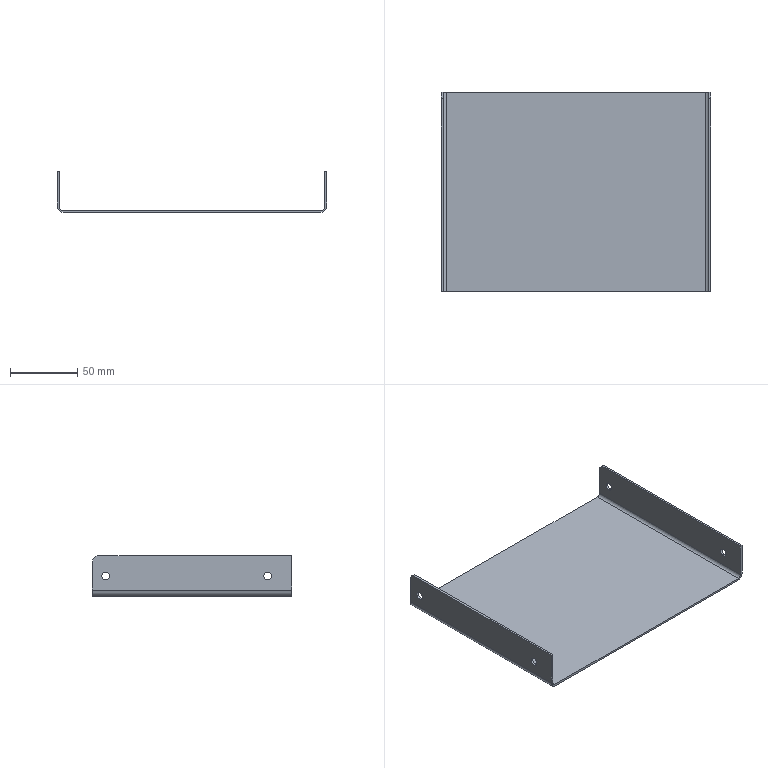Part | STEP file | [01]-11 | 1 solid | 24 faces | box 200 x 148 x 30 mm | volume 59616 mm3 | cylinder 14 | plane 10 | commonest cylinder face diameters 5.8 x8 4.6 x2 9.2 x2 10 x2